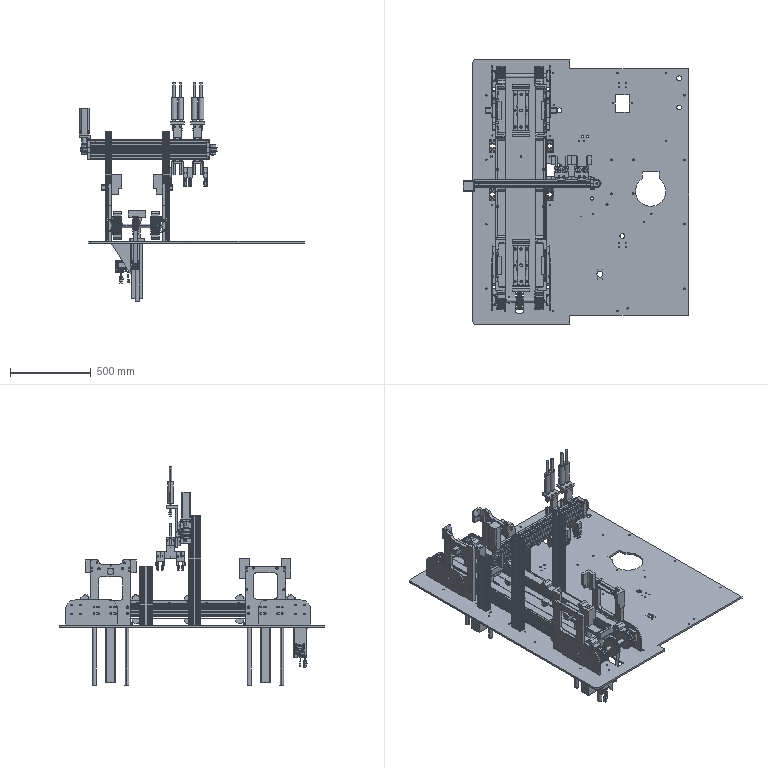Part | 193 solids | 13848 faces | volume 58138466 mm3 | plane 6387 | cylinder 5174 | spline 1490 | cone 643 | torus 126 | sphere 28 | commonest cylinder face diameters 2.5 x1318 110 x369 5 x277 6.8 x276 9 x268 3.3 x218